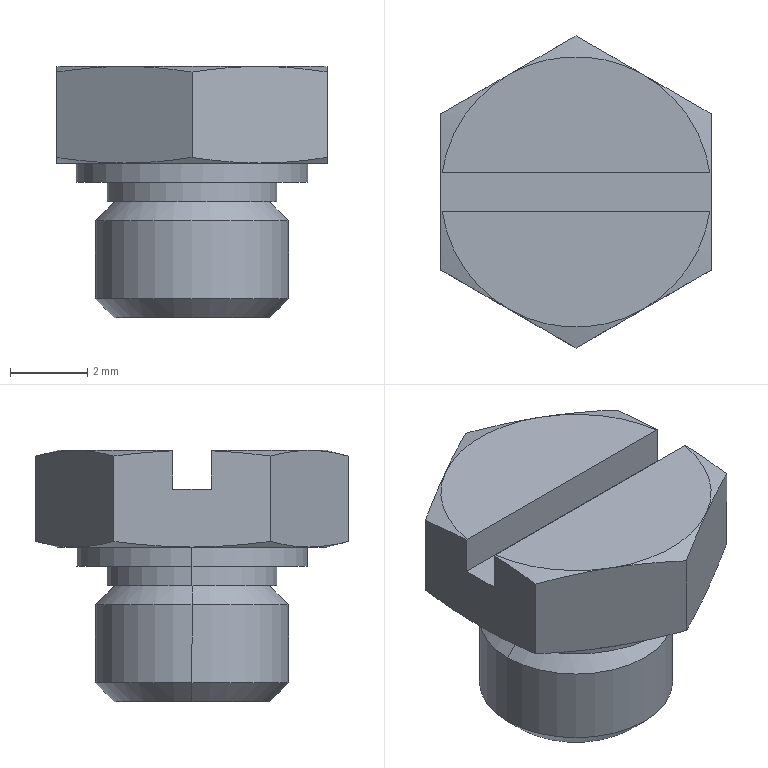Part | SolidWorks | features RefAxis 3, ICE 2, 3DProfileFeature 1, Revolution 1 | 1 solid | 37 faces | box 7 x 8.083 x 6.5 mm | volume 175.846 mm3 | cone 16 | plane 15 | cylinder 6 | commonest cylinder face diameters 4.4 x2 5 x2 6 x2
STEP:
#1=CARTESIAN_POINT('',(2.01,0.,-3.5));
#2=VERTEX_POINT('',#1);
#3=CARTESIAN_POINT('',(-2.01,0.,-3.5));
#4=VERTEX_POINT('',#3);
#5=CARTESIAN_POINT('',(0.,0.,-3.5));
#6=DIRECTION('',(0.,0.,1.));
#7=DIRECTION('',(1.,0.,0.));
#8=AXIS2_PLACEMENT_3D('',#5,#6,#7);
#9=CIRCLE('',#8,2.01);
#10=EDGE_CURVE('',#2,#4,#9,.T.);
#11=ORIENTED_EDGE('',*,*,#10,.T.);
#12=CARTESIAN_POINT('',(-2.5,0.,-3.01));
#13=VERTEX_POINT('',#12);
#14=CARTESIAN_POINT('',(-2.01,0.,-3.5));
#15=DIRECTION('',(-0.7071,0.,0.7071));
#16=VECTOR('',#15,1000.);
#17=LINE('',#14,#16);
#18=EDGE_CURVE('',#4,#13,#17,.T.);
#19=ORIENTED_EDGE('',*,*,#18,.T.);
#20=CARTESIAN_POINT('',(2.5,0.,-3.01));
#21=VERTEX_POINT('',#20);
#22=CARTESIAN_POINT('',(0.,0.,-3.01));
#23=DIRECTION('',(0.,0.,1.));
#24=DIRECTION('',(1.,0.,0.));
#25=AXIS2_PLACEMENT_3D('',#22,#23,#24);
#26=CIRCLE('',#25,2.5);
#27=EDGE_CURVE('',#21,#13,#26,.T.);
#28=ORIENTED_EDGE('',*,*,#27,.F.);
#29=CARTESIAN_POINT('',(2.01,0.,-3.5));
#30=DIRECTION('',(0.7071,0.,0.7071));
#31=VECTOR('',#30,1000.);
#32=LINE('',#29,#31);
#33=EDGE_CURVE('',#2,#21,#32,.T.);
#34=ORIENTED_EDGE('',*,*,#33,.F.);
#35=EDGE_LOOP('',(#11,#19,#28,#34));
#36=FACE_OUTER_BOUND('',#35,.T.);
#37=CARTESIAN_POINT('',(0.,0.,-3.5));
#38=DIRECTION('',(0.,0.,1.));
#39=DIRECTION('',(1.,0.,0.));
#40=AXIS2_PLACEMENT_3D('',#37,#38,#39);
#41=CONICAL_SURFACE('',#40,2.01,0.7854);
#42=ADVANCED_FACE('',(#36),#41,.T.);
#43=ORIENTED_EDGE('',*,*,#27,.T.);
#44=CARTESIAN_POINT('',(-2.5,0.,-0.9905));
#45=VERTEX_POINT('',#44);
#46=CARTESIAN_POINT('',(-2.5,0.,-3.5));
#47=DIRECTION('',(0.,0.,1.));
#48=VECTOR('',#47,1000.);
#49=LINE('',#46,#48);
#50=EDGE_CURVE('',#13,#45,#49,.T.);
#51=ORIENTED_EDGE('',*,*,#50,.T.);
#52=CARTESIAN_POINT('',(2.5,0.,-0.9905));
#53=VERTEX_POINT('',#52);
#54=CARTESIAN_POINT('',(0.,0.,-0.9905));
#55=DIRECTION('',(0.,0.,1.));
#56=DIRECTION('',(1.,0.,0.));
#57=AXIS2_PLACEMENT_3D('',#54,#55,#56);
#58=CIRCLE('',#57,2.5);
#59=EDGE_CURVE('',#53,#45,#58,.T.);
#60=ORIENTED_EDGE('',*,*,#59,.F.);
#61=CARTESIAN_POINT('',(2.5,0.,-3.5));
#62=DIRECTION('',(0.,0.,1.));
#63=VECTOR('',#62,1000.);
#64=LINE('',#61,#63);
#65=EDGE_CURVE('',#21,#53,#64,.T.);
#66=ORIENTED_EDGE('',*,*,#65,.F.);
#67=EDGE_LOOP('',(#43,#51,#60,#66));
#68=FACE_OUTER_BOUND('',#67,.T.);
#69=CARTESIAN_POINT('',(0.,0.,-3.5));
#70=DIRECTION('',(0.,0.,1.));
#71=DIRECTION('',(1.,0.,0.));
#72=AXIS2_PLACEMENT_3D('',#69,#70,#71);
#73=CYLINDRICAL_SURFACE('',#72,2.5);
#74=ADVANCED_FACE('',(#68),#73,.T.);
#75=CARTESIAN_POINT('',(2.01,0.,-0.5));
#76=VERTEX_POINT('',#75);
#77=CARTESIAN_POINT('',(-2.01,0.,-0.5));
#78=VERTEX_POINT('',#77);
#79=CARTESIAN_POINT('',(0.,0.,-0.5));
#80=DIRECTION('',(0.,0.,1.));
#81=DIRECTION('',(1.,0.,0.));
#82=AXIS2_PLACEMENT_3D('',#79,#80,#81);
#83=CIRCLE('',#82,2.01);
#84=EDGE_CURVE('',#76,#78,#83,.T.);
#85=ORIENTED_EDGE('',*,*,#84,.F.);
#86=CARTESIAN_POINT('',(2.5,0.,-0.9905));
#87=DIRECTION('',(0.7071,0.,-0.7071));
#88=VECTOR('',#87,1000.);
#89=LINE('',#86,#88);
#90=EDGE_CURVE('',#76,#53,#89,.T.);
#91=ORIENTED_EDGE('',*,*,#90,.T.);
#92=ORIENTED_EDGE('',*,*,#59,.T.);
#93=CARTESIAN_POINT('',(-2.5,0.,-0.9905));
#94=DIRECTION('',(-0.7071,0.,-0.7071));
#95=VECTOR('',#94,1000.);
#96=LINE('',#93,#95);
#97=EDGE_CURVE('',#78,#45,#96,.T.);
#98=ORIENTED_EDGE('',*,*,#97,.F.);
#99=EDGE_LOOP('',(#85,#91,#92,#98));
#100=FACE_OUTER_BOUND('',#99,.T.);
#101=CARTESIAN_POINT('',(0.,0.,-0.9905));
#102=DIRECTION('',(0.,0.,-1.));
#103=DIRECTION('',(-1.,0.,0.));
#104=AXIS2_PLACEMENT_3D('',#101,#102,#103);
#105=CONICAL_SURFACE('',#104,2.5,0.7854);
#106=ADVANCED_FACE('',(#100),#105,.T.);
#107=CARTESIAN_POINT('',(2.2,0.,-0.5));
#108=VERTEX_POINT('',#107);
#109=CARTESIAN_POINT('',(-2.2,0.,-0.5));
#110=VERTEX_POINT('',#109);
#111=CARTESIAN_POINT('',(0.,0.,-0.5));
#112=DIRECTION('',(0.,0.,1.));
#113=DIRECTION('',(1.,0.,0.));
#114=AXIS2_PLACEMENT_3D('',#111,#112,#113);
#115=CIRCLE('',#114,2.2);
#116=EDGE_CURVE('',#108,#110,#115,.T.);
#117=ORIENTED_EDGE('',*,*,#116,.T.);
#118=CARTESIAN_POINT('',(-2.2,0.,0.));
#119=VERTEX_POINT('',#118);
#120=CARTESIAN_POINT('',(-2.2,0.,-3.5));
#121=DIRECTION('',(0.,0.,1.));
#122=VECTOR('',#121,1000.);
#123=LINE('',#120,#122);
#124=EDGE_CURVE('',#110,#119,#123,.T.);
#125=ORIENTED_EDGE('',*,*,#124,.T.);
#126=CARTESIAN_POINT('',(2.2,0.,0.));
#127=VERTEX_POINT('',#126);
#128=CARTESIAN_POINT('',(0.,0.,0.));
#129=DIRECTION('',(0.,0.,1.));
#130=DIRECTION('',(1.,0.,0.));
#131=AXIS2_PLACEMENT_3D('',#128,#129,#130);
#132=CIRCLE('',#131,2.2);
#133=EDGE_CURVE('',#127,#119,#132,.T.);
#134=ORIENTED_EDGE('',*,*,#133,.F.);
#135=CARTESIAN_POINT('',(2.2,0.,-3.5));
#136=DIRECTION('',(0.,0.,1.));
#137=VECTOR('',#136,1000.);
#138=LINE('',#135,#137);
#139=EDGE_CURVE('',#108,#127,#138,.T.);
#140=ORIENTED_EDGE('',*,*,#139,.F.);
#141=EDGE_LOOP('',(#117,#125,#134,#140));
#142=FACE_OUTER_BOUND('',#141,.T.);
#143=CARTESIAN_POINT('',(0.,0.,-3.5));
#144=DIRECTION('',(0.,0.,1.));
#145=DIRECTION('',(1.,0.,0.));
#146=AXIS2_PLACEMENT_3D('',#143,#144,#145);
#147=CYLINDRICAL_SURFACE('',#146,2.2);
#148=ADVANCED_FACE('',(#142),#147,.T.);
#149=CARTESIAN_POINT('',(3.,0.,0.));
#150=VERTEX_POINT('',#149);
#151=CARTESIAN_POINT('',(-3.,0.,0.));
#152=VERTEX_POINT('',#151);
#153=CARTESIAN_POINT('',(0.,0.,0.));
#154=DIRECTION('',(0.,0.,1.));
#155=DIRECTION('',(1.,0.,0.));
#156=AXIS2_PLACEMENT_3D('',#153,#154,#155);
#157=CIRCLE('',#156,3.);
#158=EDGE_CURVE('',#150,#152,#157,.T.);
#159=ORIENTED_EDGE('',*,*,#158,.T.);
#160=CARTESIAN_POINT('',(-3.,0.,0.5));
#161=VERTEX_POINT('',#160);
#162=CARTESIAN_POINT('',(-3.,0.,-3.5));
#163=DIRECTION('',(0.,0.,1.));
#164=VECTOR('',#163,1000.);
#165=LINE('',#162,#164);
#166=EDGE_CURVE('',#152,#161,#165,.T.);
#167=ORIENTED_EDGE('',*,*,#166,.T.);
#168=CARTESIAN_POINT('',(3.,0.,0.5));
#169=VERTEX_POINT('',#168);
#170=CARTESIAN_POINT('',(0.,0.,0.5));
#171=DIRECTION('',(0.,0.,1.));
#172=DIRECTION('',(1.,0.,0.));
#173=AXIS2_PLACEMENT_3D('',#170,#171,#172);
#174=CIRCLE('',#173,3.);
#175=EDGE_CURVE('',#169,#161,#174,.T.);
#176=ORIENTED_EDGE('',*,*,#175,.F.);
#177=CARTESIAN_POINT('',(3.,0.,-3.5));
#178=DIRECTION('',(0.,0.,1.));
#179=VECTOR('',#178,1000.);
#180=LINE('',#177,#179);
#181=EDGE_CURVE('',#150,#169,#180,.T.);
#182=ORIENTED_EDGE('',*,*,#181,.F.);
#183=EDGE_LOOP('',(#159,#167,#176,#182));
#184=FACE_OUTER_BOUND('',#183,.T.);
#185=CARTESIAN_POINT('',(0.,0.,-3.5));
#186=DIRECTION('',(0.,0.,1.));
#187=DIRECTION('',(1.,0.,0.));
#188=AXIS2_PLACEMENT_3D('',#185,#186,#187);
#189=CYLINDRICAL_SURFACE('',#188,3.);
#190=ADVANCED_FACE('',(#184),#189,.T.);
#191=CARTESIAN_POINT('',(-1.75,3.031,3.));
#192=VERTEX_POINT('',#191);
#193=CARTESIAN_POINT('',(-3.464,0.5,3.));
#194=VERTEX_POINT('',#193);
#195=CARTESIAN_POINT('',(0.,0.,3.));
#196=DIRECTION('',(0.,0.,1.));
#197=DIRECTION('',(1.,0.,0.));
#198=AXIS2_PLACEMENT_3D('',#195,#196,#197);
#199=CIRCLE('',#198,3.5);
#200=EDGE_CURVE('',#192,#194,#199,.T.);
#201=ORIENTED_EDGE('',*,*,#200,.T.);
#202=CARTESIAN_POINT('',(3.464,0.5,3.));
#203=VERTEX_POINT('',#202);
#204=CARTESIAN_POINT('',(0.,0.5,3.));
#205=DIRECTION('',(1.,0.,0.));
#206=VECTOR('',#205,1000.);
#207=LINE('',#204,#206);
#208=EDGE_CURVE('',#194,#203,#207,.T.);
#209=ORIENTED_EDGE('',*,*,#208,.T.);
#210=CARTESIAN_POINT('',(1.75,3.031,3.));
#211=VERTEX_POINT('',#210);
#212=CARTESIAN_POINT('',(0.,0.,3.));
#213=DIRECTION('',(0.,0.,1.));
#214=DIRECTION('',(1.,0.,0.));
#215=AXIS2_PLACEMENT_3D('',#212,#213,#214);
#216=CIRCLE('',#215,3.5);
#217=EDGE_CURVE('',#203,#211,#216,.T.);
#218=ORIENTED_EDGE('',*,*,#217,.T.);
#219=CARTESIAN_POINT('',(0.,0.,3.));
#220=DIRECTION('',(0.,0.,1.));
#221=DIRECTION('',(1.,0.,0.));
#222=AXIS2_PLACEMENT_3D('',#219,#220,#221);
#223=CIRCLE('',#222,3.5);
#224=EDGE_CURVE('',#211,#192,#223,.T.);
#225=ORIENTED_EDGE('',*,*,#224,.T.);
#226=EDGE_LOOP('',(#201,#209,#218,#225));
#227=FACE_OUTER_BOUND('',#226,.T.);
#228=CARTESIAN_POINT('',(0.,0.,3.));
#229=DIRECTION('',(0.,0.,-1.));
#230=DIRECTION('',(-1.,0.,0.));
#231=AXIS2_PLACEMENT_3D('',#228,#229,#230);
#232=PLANE('',#231);
#233=ADVANCED_FACE('',(#227),#232,.F.);
#234=CARTESIAN_POINT('',(1.75,-3.031,0.5));
#235=VERTEX_POINT('',#234);
#236=CARTESIAN_POINT('',(0.,-4.041,0.6451));
#237=VERTEX_POINT('',#236);
#238=CARTESIAN_POINT('',(1.75,-3.031,0.5));
#239=CARTESIAN_POINT('',(1.167,-3.368,0.5));
#240=CARTESIAN_POINT('',(0.5833,-3.705,0.5548));
#241=CARTESIAN_POINT('',(0.,-4.041,0.6451));
#242=B_SPLINE_CURVE_WITH_KNOTS('',3,(#238,#239,#240,#241),.UNSPECIFIED.,.F.,.F.,(4,4),(0.002021,0.004042),.UNSPECIFIED.);
#243=EDGE_CURVE('',#235,#237,#242,.T.);
#244=ORIENTED_EDGE('',*,*,#243,.T.);
#245=CARTESIAN_POINT('',(-1.75,-3.031,0.5));
#246=VERTEX_POINT('',#245);
#247=CARTESIAN_POINT('',(0.,-4.041,0.6451));
#248=CARTESIAN_POINT('',(-0.5833,-3.705,0.5548));
#249=CARTESIAN_POINT('',(-1.167,-3.368,0.5));
#250=CARTESIAN_POINT('',(-1.75,-3.031,0.5));
#251=B_SPLINE_CURVE_WITH_KNOTS('',3,(#247,#248,#249,#250),.UNSPECIFIED.,.F.,.F.,(4,4),(0.000000231,0.002021),.UNSPECIFIED.);
#252=EDGE_CURVE('',#237,#246,#251,.T.);
#253=ORIENTED_EDGE('',*,*,#252,.T.);
#254=CARTESIAN_POINT('',(0.,0.,0.5));
#255=DIRECTION('',(0.,0.,1.));
#256=DIRECTION('',(1.,0.,0.));
#257=AXIS2_PLACEMENT_3D('',#254,#255,#256);
#258=CIRCLE('',#257,3.5);
#259=EDGE_CURVE('',#246,#235,#258,.T.);
#260=ORIENTED_EDGE('',*,*,#259,.T.);
#261=EDGE_LOOP('',(#244,#253,#260));
#262=FACE_OUTER_BOUND('',#261,.T.);
#263=CARTESIAN_POINT('',(0.,0.,0.5));
#264=DIRECTION('',(0.,0.,1.));
#265=DIRECTION('',(1.,0.,0.));
#266=AXIS2_PLACEMENT_3D('',#263,#264,#265);
#267=CONICAL_SURFACE('',#266,3.5,1.309);
#268=ADVANCED_FACE('',(#262),#267,.T.);
#269=CARTESIAN_POINT('',(-3.5,0.,0.5));
#270=VERTEX_POINT('',#269);
#271=CARTESIAN_POINT('',(0.,0.,0.5));
#272=DIRECTION('',(0.,0.,1.));
#273=DIRECTION('',(1.,0.,0.));
#274=AXIS2_PLACEMENT_3D('',#271,#272,#273);
#275=CIRCLE('',#274,3.5);
#276=EDGE_CURVE('',#270,#246,#275,.T.);
#277=ORIENTED_EDGE('',*,*,#276,.T.);
#278=CARTESIAN_POINT('',(-3.5,-2.021,0.6451));
#279=VERTEX_POINT('',#278);
#280=CARTESIAN_POINT('',(-1.75,-3.031,0.5));
#281=CARTESIAN_POINT('',(-2.333,-2.694,0.5));
#282=CARTESIAN_POINT('',(-2.917,-2.358,0.5548));
#283=CARTESIAN_POINT('',(-3.5,-2.021,0.6451));
#284=B_SPLINE_CURVE_WITH_KNOTS('',3,(#280,#281,#282,#283),.UNSPECIFIED.,.F.,.F.,(4,4),(0.002021,0.004042),.UNSPECIFIED.);
#285=EDGE_CURVE('',#246,#279,#284,.T.);
#286=ORIENTED_EDGE('',*,*,#285,.T.);
#287=CARTESIAN_POINT('',(-3.5,-2.021,0.6451));
#288=CARTESIAN_POINT('',(-3.5,-1.349,0.5551));
#289=CARTESIAN_POINT('',(-3.5,-0.6727,0.5));
#290=CARTESIAN_POINT('',(-3.5,0.,0.5));
#291=B_SPLINE_CURVE_WITH_KNOTS('',3,(#287,#288,#289,#290),.UNSPECIFIED.,.F.,.F.,(4,4),(0.0034,0.00543),.UNSPECIFIED.);
#292=EDGE_CURVE('',#279,#270,#291,.T.);
#293=ORIENTED_EDGE('',*,*,#292,.T.);
#294=EDGE_LOOP('',(#277,#286,#293));
#295=FACE_OUTER_BOUND('',#294,.T.);
#296=CARTESIAN_POINT('',(0.,0.,0.5));
#297=DIRECTION('',(0.,0.,1.));
#298=DIRECTION('',(1.,0.,0.));
#299=AXIS2_PLACEMENT_3D('',#296,#297,#298);
#300=CONICAL_SURFACE('',#299,3.5,1.309);
#301=ADVANCED_FACE('',(#295),#300,.T.);
#302=CARTESIAN_POINT('',(-1.75,3.031,0.5));
#303=VERTEX_POINT('',#302);
#304=CARTESIAN_POINT('',(0.,0.,0.5));
#305=DIRECTION('',(0.,0.,1.));
#306=DIRECTION('',(1.,0.,0.));
#307=AXIS2_PLACEMENT_3D('',#304,#305,#306);
#308=CIRCLE('',#307,3.5);
#309=EDGE_CURVE('',#303,#270,#308,.T.);
#310=ORIENTED_EDGE('',*,*,#309,.T.);
#311=CARTESIAN_POINT('',(-3.5,2.021,0.6451));
#312=VERTEX_POINT('',#311);
#313=CARTESIAN_POINT('',(-3.5,0.,0.5));
#314=CARTESIAN_POINT('',(-3.5,0.675,0.5));
#315=CARTESIAN_POINT('',(-3.5,1.348,0.555));
#316=CARTESIAN_POINT('',(-3.5,2.021,0.6451));
#317=B_SPLINE_CURVE_WITH_KNOTS('',3,(#313,#314,#315,#316),.UNSPECIFIED.,.F.,.F.,(4,4),(0.00543,0.007468),.UNSPECIFIED.);
#318=EDGE_CURVE('',#270,#312,#317,.T.);
#319=ORIENTED_EDGE('',*,*,#318,.T.);
#320=CARTESIAN_POINT('',(-3.5,2.021,0.6451));
#321=CARTESIAN_POINT('',(-2.917,2.358,0.5548));
#322=CARTESIAN_POINT('',(-2.333,2.694,0.5));
#323=CARTESIAN_POINT('',(-1.75,3.031,0.5));
#324=B_SPLINE_CURVE_WITH_KNOTS('',3,(#320,#321,#322,#323),.UNSPECIFIED.,.F.,.F.,(4,4),(0.000000231,0.002021),.UNSPECIFIED.);
#325=EDGE_CURVE('',#312,#303,#324,.T.);
#326=ORIENTED_EDGE('',*,*,#325,.T.);
#327=EDGE_LOOP('',(#310,#319,#326));
#328=FACE_OUTER_BOUND('',#327,.T.);
#329=CARTESIAN_POINT('',(0.,0.,0.5));
#330=DIRECTION('',(0.,0.,1.));
#331=DIRECTION('',(1.,0.,0.));
#332=AXIS2_PLACEMENT_3D('',#329,#330,#331);
#333=CONICAL_SURFACE('',#332,3.5,1.309);
#334=ADVANCED_FACE('',(#328),#333,.T.);
#335=CARTESIAN_POINT('',(3.5,0.,0.5));
#336=VERTEX_POINT('',#335);
#337=CARTESIAN_POINT('',(3.5,-2.021,0.6451));
#338=VERTEX_POINT('',#337);
#339=CARTESIAN_POINT('',(3.5,0.,0.5));
#340=CARTESIAN_POINT('',(3.5,-0.6727,0.5));
#341=CARTESIAN_POINT('',(3.5,-1.349,0.5551));
#342=CARTESIAN_POINT('',(3.5,-2.021,0.6451));
#343=B_SPLINE_CURVE_WITH_KNOTS('',3,(#339,#340,#341,#342),.UNSPECIFIED.,.F.,.F.,(4,4),(0.0098,0.01183),.UNSPECIFIED.);
#344=EDGE_CURVE('',#336,#338,#343,.T.);
#345=ORIENTED_EDGE('',*,*,#344,.T.);
#346=CARTESIAN_POINT('',(3.5,-2.021,0.6451));
#347=CARTESIAN_POINT('',(2.917,-2.358,0.5548));
#348=CARTESIAN_POINT('',(2.333,-2.694,0.5));
#349=CARTESIAN_POINT('',(1.75,-3.031,0.5));
#350=B_SPLINE_CURVE_WITH_KNOTS('',3,(#346,#347,#348,#349),.UNSPECIFIED.,.F.,.F.,(4,4),(0.000000231,0.002021),.UNSPECIFIED.);
#351=EDGE_CURVE('',#338,#235,#350,.T.);
#352=ORIENTED_EDGE('',*,*,#351,.T.);
#353=CARTESIAN_POINT('',(0.,0.,0.5));
#354=DIRECTION('',(0.,0.,1.));
#355=DIRECTION('',(1.,0.,0.));
#356=AXIS2_PLACEMENT_3D('',#353,#354,#355);
#357=CIRCLE('',#356,3.5);
#358=EDGE_CURVE('',#235,#336,#357,.T.);
#359=ORIENTED_EDGE('',*,*,#358,.T.);
#360=EDGE_LOOP('',(#345,#352,#359));
#361=FACE_OUTER_BOUND('',#360,.T.);
#362=CARTESIAN_POINT('',(0.,0.,0.5));
#363=DIRECTION('',(0.,0.,1.));
#364=DIRECTION('',(1.,0.,0.));
#365=AXIS2_PLACEMENT_3D('',#362,#363,#364);
#366=CONICAL_SURFACE('',#365,3.5,1.309);
#367=ADVANCED_FACE('',(#361),#366,.T.);
#368=CARTESIAN_POINT('',(1.75,3.031,0.5));
#369=VERTEX_POINT('',#368);
#370=CARTESIAN_POINT('',(0.,0.,0.5));
#371=DIRECTION('',(0.,0.,1.));
#372=DIRECTION('',(1.,0.,0.));
#373=AXIS2_PLACEMENT_3D('',#370,#371,#372);
#374=CIRCLE('',#373,3.5);
#375=EDGE_CURVE('',#369,#303,#374,.T.);
#376=ORIENTED_EDGE('',*,*,#375,.T.);
#377=CARTESIAN_POINT('',(0.,4.041,0.6451));
#378=VERTEX_POINT('',#377);
#379=CARTESIAN_POINT('',(-1.75,3.031,0.5));
#380=CARTESIAN_POINT('',(-1.167,3.368,0.5));
#381=CARTESIAN_POINT('',(-0.5833,3.705,0.5548));
#382=CARTESIAN_POINT('',(0.,4.041,0.6451));
#383=B_SPLINE_CURVE_WITH_KNOTS('',3,(#379,#380,#381,#382),.UNSPECIFIED.,.F.,.F.,(4,4),(0.002021,0.004042),.UNSPECIFIED.);
#384=EDGE_CURVE('',#303,#378,#383,.T.);
#385=ORIENTED_EDGE('',*,*,#384,.T.);
#386=CARTESIAN_POINT('',(0.,4.041,0.6451));
#387=CARTESIAN_POINT('',(0.5833,3.705,0.5548));
#388=CARTESIAN_POINT('',(1.167,3.368,0.5));
#389=CARTESIAN_POINT('',(1.75,3.031,0.5));
#390=B_SPLINE_CURVE_WITH_KNOTS('',3,(#386,#387,#388,#389),.UNSPECIFIED.,.F.,.F.,(4,4),(0.000000231,0.002021),.UNSPECIFIED.);
#391=EDGE_CURVE('',#378,#369,#390,.T.);
#392=ORIENTED_EDGE('',*,*,#391,.T.);
#393=EDGE_LOOP('',(#376,#385,#392));
#394=FACE_OUTER_BOUND('',#393,.T.);
#395=CARTESIAN_POINT('',(0.,0.,0.5));
#396=DIRECTION('',(0.,0.,1.));
#397=DIRECTION('',(1.,0.,0.));
#398=AXIS2_PLACEMENT_3D('',#395,#396,#397);
#399=CONICAL_SURFACE('',#398,3.5,1.309);
#400=ADVANCED_FACE('',(#394),#399,.T.);
#401=CARTESIAN_POINT('',(3.5,2.021,0.6451));
#402=VERTEX_POINT('',#401);
#403=CARTESIAN_POINT('',(1.75,3.031,0.5));
#404=CARTESIAN_POINT('',(2.333,2.694,0.5));
#405=CARTESIAN_POINT('',(2.917,2.358,0.5548));
#406=CARTESIAN_POINT('',(3.5,2.021,0.6451));
#407=B_SPLINE_CURVE_WITH_KNOTS('',3,(#403,#404,#405,#406),.UNSPECIFIED.,.F.,.F.,(4,4),(0.002021,0.004042),.UNSPECIFIED.);
#408=EDGE_CURVE('',#369,#402,#407,.T.);
#409=ORIENTED_EDGE('',*,*,#408,.T.);
#410=CARTESIAN_POINT('',(3.5,2.021,0.6451));
#411=CARTESIAN_POINT('',(3.5,1.348,0.555));
#412=CARTESIAN_POINT('',(3.5,0.675,0.5));
#413=CARTESIAN_POINT('',(3.5,0.,0.5));
#414=B_SPLINE_CURVE_WITH_KNOTS('',3,(#410,#411,#412,#413),.UNSPECIFIED.,.F.,.F.,(4,4),(0.007765,0.0098),.UNSPECIFIED.);
#415=EDGE_CURVE('',#402,#336,#414,.T.);
#416=ORIENTED_EDGE('',*,*,#415,.T.);
#417=CARTESIAN_POINT('',(0.,0.,0.5));
#418=DIRECTION('',(0.,0.,1.));
#419=DIRECTION('',(1.,0.,0.));
#420=AXIS2_PLACEMENT_3D('',#417,#418,#419);
#421=CIRCLE('',#420,3.5);
#422=EDGE_CURVE('',#336,#369,#421,.T.);
#423=ORIENTED_EDGE('',*,*,#422,.T.);
#424=EDGE_LOOP('',(#409,#416,#423));
#425=FACE_OUTER_BOUND('',#424,.T.);
#426=CARTESIAN_POINT('',(0.,0.,0.5));
#427=DIRECTION('',(0.,0.,1.));
#428=DIRECTION('',(1.,0.,0.));
#429=AXIS2_PLACEMENT_3D('',#426,#427,#428);
#430=CONICAL_SURFACE('',#429,3.5,1.309);
#431=ADVANCED_FACE('',(#425),#430,.T.);
#432=ORIENTED_EDGE('',*,*,#422,.F.);
#433=ORIENTED_EDGE('',*,*,#358,.F.);
#434=ORIENTED_EDGE('',*,*,#259,.F.);
#435=ORIENTED_EDGE('',*,*,#276,.F.);
#436=ORIENTED_EDGE('',*,*,#309,.F.);
#437=ORIENTED_EDGE('',*,*,#375,.F.);
#438=EDGE_LOOP('',(#432,#433,#434,#435,#436,#437));
#439=FACE_OUTER_BOUND('',#438,.T.);
#440=ORIENTED_EDGE('',*,*,#175,.T.);
#441=CARTESIAN_POINT('',(0.,0.,0.5));
#442=DIRECTION('',(0.,0.,1.));
#443=DIRECTION('',(1.,0.,0.));
#444=AXIS2_PLACEMENT_3D('',#441,#442,#443);
#445=CIRCLE('',#444,3.);
#446=EDGE_CURVE('',#161,#169,#445,.T.);
#447=ORIENTED_EDGE('',*,*,#446,.T.);
#448=EDGE_LOOP('',(#440,#447));
#449=FACE_BOUND('',#448,.T.);
#450=CARTESIAN_POINT('',(0.,3.5,0.5));
#451=DIRECTION('',(0.,0.,1.));
#452=DIRECTION('',(1.,0.,0.));
#453=AXIS2_PLACEMENT_3D('',#450,#451,#452);
#454=PLANE('',#453);
#455=ADVANCED_FACE('',(#439,#449),#454,.F.);
#456=ORIENTED_EDGE('',*,*,#166,.F.);
#457=CARTESIAN_POINT('',(0.,0.,0.));
#458=DIRECTION('',(0.,0.,1.));
#459=DIRECTION('',(1.,0.,0.));
#460=AXIS2_PLACEMENT_3D('',#457,#458,#459);
#461=CIRCLE('',#460,3.);
#462=EDGE_CURVE('',#152,#150,#461,.T.);
#463=ORIENTED_EDGE('',*,*,#462,.T.);
#464=ORIENTED_EDGE('',*,*,#181,.T.);
#465=ORIENTED_EDGE('',*,*,#446,.F.);
#466=EDGE_LOOP('',(#456,#463,#464,#465));
#467=FACE_OUTER_BOUND('',#466,.T.);
#468=CARTESIAN_POINT('',(0.,0.,-3.5));
#469=DIRECTION('',(0.,0.,1.));
#470=DIRECTION('',(1.,0.,0.));
#471=AXIS2_PLACEMENT_3D('',#468,#469,#470);
#472=CYLINDRICAL_SURFACE('',#471,3.);
#473=ADVANCED_FACE('',(#467),#472,.T.);
#474=ORIENTED_EDGE('',*,*,#158,.F.);
#475=ORIENTED_EDGE('',*,*,#462,.F.);
#476=EDGE_LOOP('',(#474,#475));
#477=FACE_OUTER_BOUND('',#476,.T.);
#478=ORIENTED_EDGE('',*,*,#133,.T.);
#479=CARTESIAN_POINT('',(0.,0.,0.));
#480=DIRECTION('',(0.,0.,1.));
#481=DIRECTION('',(1.,0.,0.));
#482=AXIS2_PLACEMENT_3D('',#479,#480,#481);
#483=CIRCLE('',#482,2.2);
#484=EDGE_CURVE('',#119,#127,#483,.T.);
#485=ORIENTED_EDGE('',*,*,#484,.T.);
#486=EDGE_LOOP('',(#478,#485));
#487=FACE_BOUND('',#486,.T.);
#488=CARTESIAN_POINT('',(0.,3.,0.));
#489=DIRECTION('',(0.,0.,1.));
#490=DIRECTION('',(1.,0.,0.));
#491=AXIS2_PLACEMENT_3D('',#488,#489,#490);
#492=PLANE('',#491);
#493=ADVANCED_FACE('',(#477,#487),#492,.F.);
#494=ORIENTED_EDGE('',*,*,#124,.F.);
#495=CARTESIAN_POINT('',(0.,0.,-0.5));
#496=DIRECTION('',(0.,0.,1.));
#497=DIRECTION('',(1.,0.,0.));
#498=AXIS2_PLACEMENT_3D('',#495,#496,#497);
#499=CIRCLE('',#498,2.2);
#500=EDGE_CURVE('',#110,#108,#499,.T.);
#501=ORIENTED_EDGE('',*,*,#500,.T.);
#502=ORIENTED_EDGE('',*,*,#139,.T.);
#503=ORIENTED_EDGE('',*,*,#484,.F.);
#504=EDGE_LOOP('',(#494,#501,#502,#503));
#505=FACE_OUTER_BOUND('',#504,.T.);
#506=CARTESIAN_POINT('',(0.,0.,-3.5));
#507=DIRECTION('',(0.,0.,1.));
#508=DIRECTION('',(1.,0.,0.));
#509=AXIS2_PLACEMENT_3D('',#506,#507,#508);
#510=CYLINDRICAL_SURFACE('',#509,2.2);
#511=ADVANCED_FACE('',(#505),#510,.T.);
#512=ORIENTED_EDGE('',*,*,#116,.F.);
#513=ORIENTED_EDGE('',*,*,#500,.F.);
#514=EDGE_LOOP('',(#512,#513));
#515=FACE_OUTER_BOUND('',#514,.T.);
#516=CARTESIAN_POINT('',(0.,0.,-0.5));
#517=DIRECTION('',(0.,0.,1.));
#518=DIRECTION('',(1.,0.,0.));
#519=AXIS2_PLACEMENT_3D('',#516,#517,#518);
#520=CIRCLE('',#519,2.01);
#521=EDGE_CURVE('',#78,#76,#520,.T.);
#522=ORIENTED_EDGE('',*,*,#521,.T.);
#523=ORIENTED_EDGE('',*,*,#84,.T.);
#524=EDGE_LOOP('',(#522,#523));
#525=FACE_BOUND('',#524,.T.);
#526=CARTESIAN_POINT('',(0.,2.2,-0.5));
#527=DIRECTION('',(0.,0.,1.));
#528=DIRECTION('',(1.,0.,0.));
#529=AXIS2_PLACEMENT_3D('',#526,#527,#528);
#530=PLANE('',#529);
#531=ADVANCED_FACE('',(#515,#525),#530,.F.);
#532=ORIENTED_EDGE('',*,*,#90,.F.);
#533=ORIENTED_EDGE('',*,*,#521,.F.);
#534=ORIENTED_EDGE('',*,*,#97,.T.);
#535=CARTESIAN_POINT('',(0.,0.,-0.9905));
#536=DIRECTION('',(0.,0.,1.));
#537=DIRECTION('',(1.,0.,0.));
#538=AXIS2_PLACEMENT_3D('',#535,#536,#537);
#539=CIRCLE('',#538,2.5);
#540=EDGE_CURVE('',#45,#53,#539,.T.);
#541=ORIENTED_EDGE('',*,*,#540,.T.);
#542=EDGE_LOOP('',(#532,#533,#534,#541));
#543=FACE_OUTER_BOUND('',#542,.T.);
#544=CARTESIAN_POINT('',(0.,0.,-0.9905));
#545=DIRECTION('',(0.,0.,-1.));
#546=DIRECTION('',(-1.,0.,0.));
#547=AXIS2_PLACEMENT_3D('',#544,#545,#546);
#548=CONICAL_SURFACE('',#547,2.5,0.7854);
#549=ADVANCED_FACE('',(#543),#548,.T.);
#550=ORIENTED_EDGE('',*,*,#50,.F.);
#551=CARTESIAN_POINT('',(0.,0.,-3.01));
#552=DIRECTION('',(0.,0.,1.));
#553=DIRECTION('',(1.,0.,0.));
#554=AXIS2_PLACEMENT_3D('',#551,#552,#553);
#555=CIRCLE('',#554,2.5);
#556=EDGE_CURVE('',#13,#21,#555,.T.);
#557=ORIENTED_EDGE('',*,*,#556,.T.);
#558=ORIENTED_EDGE('',*,*,#65,.T.);
#559=ORIENTED_EDGE('',*,*,#540,.F.);
#560=EDGE_LOOP('',(#550,#557,#558,#559));
#561=FACE_OUTER_BOUND('',#560,.T.);
#562=CARTESIAN_POINT('',(0.,0.,-3.5));
#563=DIRECTION('',(0.,0.,1.));
#564=DIRECTION('',(1.,0.,0.));
#565=AXIS2_PLACEMENT_3D('',#562,#563,#564);
#566=CYLINDRICAL_SURFACE('',#565,2.5);
#567=ADVANCED_FACE('',(#561),#566,.T.);
#568=ORIENTED_EDGE('',*,*,#18,.F.);
#569=CARTESIAN_POINT('',(0.,0.,-3.5));
#570=DIRECTION('',(0.,0.,1.));
#571=DIRECTION('',(1.,0.,0.));
#572=AXIS2_PLACEMENT_3D('',#569,#570,#571);
#573=CIRCLE('',#572,2.01);
#574=EDGE_CURVE('',#4,#2,#573,.T.);
#575=ORIENTED_EDGE('',*,*,#574,.T.);
#576=ORIENTED_EDGE('',*,*,#33,.T.);
#577=ORIENTED_EDGE('',*,*,#556,.F.);
#578=EDGE_LOOP('',(#568,#575,#576,#577));
#579=FACE_OUTER_BOUND('',#578,.T.);
#580=CARTESIAN_POINT('',(0.,0.,-3.5));
#581=DIRECTION('',(0.,0.,1.));
#582=DIRECTION('',(1.,0.,0.));
#583=AXIS2_PLACEMENT_3D('',#580,#581,#582);
#584=CONICAL_SURFACE('',#583,2.01,0.7854);
#585=ADVANCED_FACE('',(#579),#584,.T.);
#586=ORIENTED_EDGE('',*,*,#10,.F.);
#587=ORIENTED_EDGE('',*,*,#574,.F.);
#588=EDGE_LOOP('',(#586,#587));
#589=FACE_OUTER_BOUND('',#588,.T.);
#590=CARTESIAN_POINT('',(0.,2.01,-3.5));
#591=DIRECTION('',(0.,0.,1.));
#592=DIRECTION('',(1.,0.,0.));
#593=AXIS2_PLACEMENT_3D('',#590,#591,#592);
#594=PLANE('',#593);
#595=ADVANCED_FACE('',(#589),#594,.F.);
#596=CARTESIAN_POINT('',(0.,4.041,2.855));
#597=VERTEX_POINT('',#596);
#598=CARTESIAN_POINT('',(0.,4.041,3.));
#599=DIRECTION('',(0.,0.,-1.));
#600=VECTOR('',#599,1000.);
#601=LINE('',#598,#600);
#602=EDGE_CURVE('',#597,#378,#601,.T.);
#603=ORIENTED_EDGE('',*,*,#602,.T.);
#604=ORIENTED_EDGE('',*,*,#384,.F.);
#605=ORIENTED_EDGE('',*,*,#325,.F.);
#606=CARTESIAN_POINT('',(-3.5,2.021,2.855));
#607=VERTEX_POINT('',#606);
#608=CARTESIAN_POINT('',(-3.5,2.021,3.));
#609=DIRECTION('',(0.,0.,-1.));
#610=VECTOR('',#609,1000.);
#611=LINE('',#608,#610);
#612=EDGE_CURVE('',#607,#312,#611,.T.);
#613=ORIENTED_EDGE('',*,*,#612,.F.);
#614=CARTESIAN_POINT('',(-1.75,3.031,3.));
#615=CARTESIAN_POINT('',(-2.333,2.694,3.));
#616=CARTESIAN_POINT('',(-2.917,2.358,2.945));
#617=CARTESIAN_POINT('',(-3.5,2.021,2.855));
#618=B_SPLINE_CURVE_WITH_KNOTS('',3,(#614,#615,#616,#617),.UNSPECIFIED.,.F.,.F.,(4,4),(0.002021,0.004042),.UNSPECIFIED.);
#619=EDGE_CURVE('',#192,#607,#618,.T.);
#620=ORIENTED_EDGE('',*,*,#619,.F.);
#621=CARTESIAN_POINT('',(0.,4.041,2.855));
#622=CARTESIAN_POINT('',(-0.5833,3.705,2.945));
#623=CARTESIAN_POINT('',(-1.167,3.368,3.));
#624=CARTESIAN_POINT('',(-1.75,3.031,3.));
#625=B_SPLINE_CURVE_WITH_KNOTS('',3,(#621,#622,#623,#624),.UNSPECIFIED.,.F.,.F.,(4,4),(0.000000231,0.002021),.UNSPECIFIED.);
#626=EDGE_CURVE('',#597,#192,#625,.T.);
#627=ORIENTED_EDGE('',*,*,#626,.F.);
#628=EDGE_LOOP('',(#603,#604,#605,#613,#620,#627));
#629=FACE_OUTER_BOUND('',#628,.T.);
#630=CARTESIAN_POINT('',(0.,4.041,3.));
#631=DIRECTION('',(0.5,-0.866,0.));
#632=DIRECTION('',(0.866,0.5,0.));
#633=AXIS2_PLACEMENT_3D('',#630,#631,#632);
#634=PLANE('',#633);
#635=ADVANCED_FACE('',(#629),#634,.F.);
#636=CARTESIAN_POINT('',(-3.5,0.5,2.));
#637=VERTEX_POINT('',#636);
#638=CARTESIAN_POINT('',(-3.5,-0.5,2.));
#639=VERTEX_POINT('',#638);
#640=CARTESIAN_POINT('',(-3.5,2.021,2.));
#641=DIRECTION('',(0.,-1.,0.));
#642=VECTOR('',#641,1000.);
#643=LINE('',#640,#642);
#644=EDGE_CURVE('',#637,#639,#643,.T.);
#645=ORIENTED_EDGE('',*,*,#644,.F.);
#646=CARTESIAN_POINT('',(-3.5,0.5,2.99));
#647=VERTEX_POINT('',#646);
#648=CARTESIAN_POINT('',(-3.5,0.5,3.));
#649=DIRECTION('',(0.,0.,1.));
#650=VECTOR('',#649,1000.);
#651=LINE('',#648,#650);
#652=EDGE_CURVE('',#637,#647,#651,.T.);
#653=ORIENTED_EDGE('',*,*,#652,.T.);
#654=CARTESIAN_POINT('',(-3.5,2.021,2.855));
#655=CARTESIAN_POINT('',(-3.5,1.514,2.923));
#656=CARTESIAN_POINT('',(-3.5,1.008,2.971));
#657=CARTESIAN_POINT('',(-3.5,0.5,2.99));
#658=B_SPLINE_CURVE_WITH_KNOTS('',3,(#654,#655,#656,#657),.UNSPECIFIED.,.F.,.F.,(4,4),(0.007765,0.009297),.UNSPECIFIED.);
#659=EDGE_CURVE('',#607,#647,#658,.T.);
#660=ORIENTED_EDGE('',*,*,#659,.F.);
#661=ORIENTED_EDGE('',*,*,#612,.T.);
#662=ORIENTED_EDGE('',*,*,#318,.F.);
#663=ORIENTED_EDGE('',*,*,#292,.F.);
#664=CARTESIAN_POINT('',(-3.5,-2.021,2.855));
#665=VERTEX_POINT('',#664);
#666=CARTESIAN_POINT('',(-3.5,-2.021,3.));
#667=DIRECTION('',(0.,0.,-1.));
#668=VECTOR('',#667,1000.);
#669=LINE('',#666,#668);
#670=EDGE_CURVE('',#665,#279,#669,.T.);
#671=ORIENTED_EDGE('',*,*,#670,.F.);
#672=CARTESIAN_POINT('',(-3.5,-0.5,2.99));
#673=VERTEX_POINT('',#672);
#674=CARTESIAN_POINT('',(-3.5,-0.5,2.99));
#675=CARTESIAN_POINT('',(-3.5,-1.007,2.971));
#676=CARTESIAN_POINT('',(-3.5,-1.515,2.923));
#677=CARTESIAN_POINT('',(-3.5,-2.021,2.855));
#678=B_SPLINE_CURVE_WITH_KNOTS('',3,(#674,#675,#676,#677),.UNSPECIFIED.,.F.,.F.,(4,4),(0.0103,0.01183),.UNSPECIFIED.);
#679=EDGE_CURVE('',#673,#665,#678,.T.);
#680=ORIENTED_EDGE('',*,*,#679,.F.);
#681=CARTESIAN_POINT('',(-3.5,-0.5,3.));
#682=DIRECTION('',(0.,0.,-1.));
#683=VECTOR('',#682,1000.);
#684=LINE('',#681,#683);
#685=EDGE_CURVE('',#673,#639,#684,.T.);
#686=ORIENTED_EDGE('',*,*,#685,.T.);
#687=EDGE_LOOP('',(#645,#653,#660,#661,#662,#663,#671,#680,#686));
#688=FACE_OUTER_BOUND('',#687,.T.);
#689=CARTESIAN_POINT('',(-3.5,2.021,3.));
#690=DIRECTION('',(1.,0.,0.));
#691=DIRECTION('',(0.,0.,-1.));
#692=AXIS2_PLACEMENT_3D('',#689,#690,#691);
#693=PLANE('',#692);
#694=ADVANCED_FACE('',(#688),#693,.F.);
#695=ORIENTED_EDGE('',*,*,#670,.T.);
#696=ORIENTED_EDGE('',*,*,#285,.F.);
#697=ORIENTED_EDGE('',*,*,#252,.F.);
#698=CARTESIAN_POINT('',(0.,-4.041,2.855));
#699=VERTEX_POINT('',#698);
#700=CARTESIAN_POINT('',(0.,-4.041,3.));
#701=DIRECTION('',(0.,0.,-1.));
#702=VECTOR('',#701,1000.);
#703=LINE('',#700,#702);
#704=EDGE_CURVE('',#699,#237,#703,.T.);
#705=ORIENTED_EDGE('',*,*,#704,.F.);
#706=CARTESIAN_POINT('',(-1.75,-3.031,3.));
#707=VERTEX_POINT('',#706);
#708=CARTESIAN_POINT('',(-1.75,-3.031,3.));
#709=CARTESIAN_POINT('',(-1.167,-3.368,3.));
#710=CARTESIAN_POINT('',(-0.5833,-3.705,2.945));
#711=CARTESIAN_POINT('',(0.,-4.041,2.855));
#712=B_SPLINE_CURVE_WITH_KNOTS('',3,(#708,#709,#710,#711),.UNSPECIFIED.,.F.,.F.,(4,4),(0.002021,0.004042),.UNSPECIFIED.);
#713=EDGE_CURVE('',#707,#699,#712,.T.);
#714=ORIENTED_EDGE('',*,*,#713,.F.);
#715=CARTESIAN_POINT('',(-3.5,-2.021,2.855));
#716=CARTESIAN_POINT('',(-2.917,-2.358,2.945));
#717=CARTESIAN_POINT('',(-2.333,-2.694,3.));
#718=CARTESIAN_POINT('',(-1.75,-3.031,3.));
#719=B_SPLINE_CURVE_WITH_KNOTS('',3,(#715,#716,#717,#718),.UNSPECIFIED.,.F.,.F.,(4,4),(0.000000231,0.002021),.UNSPECIFIED.);
#720=EDGE_CURVE('',#665,#707,#719,.T.);
#721=ORIENTED_EDGE('',*,*,#720,.F.);
#722=EDGE_LOOP('',(#695,#696,#697,#705,#714,#721));
#723=FACE_OUTER_BOUND('',#722,.T.);
#724=CARTESIAN_POINT('',(-3.5,-2.021,3.));
#725=DIRECTION('',(0.5,0.866,0.));
#726=DIRECTION('',(-0.866,0.5,0.));
#727=AXIS2_PLACEMENT_3D('',#724,#725,#726);
#728=PLANE('',#727);
#729=ADVANCED_FACE('',(#723),#728,.F.);
#730=ORIENTED_EDGE('',*,*,#704,.T.);
#731=ORIENTED_EDGE('',*,*,#243,.F.);
#732=ORIENTED_EDGE('',*,*,#351,.F.);
#733=CARTESIAN_POINT('',(3.5,-2.021,2.855));
#734=VERTEX_POINT('',#733);
#735=CARTESIAN_POINT('',(3.5,-2.021,3.));
#736=DIRECTION('',(0.,0.,-1.));
#737=VECTOR('',#736,1000.);
#738=LINE('',#735,#737);
#739=EDGE_CURVE('',#734,#338,#738,.T.);
#740=ORIENTED_EDGE('',*,*,#739,.F.);
#741=CARTESIAN_POINT('',(1.75,-3.031,3.));
#742=VERTEX_POINT('',#741);
#743=CARTESIAN_POINT('',(1.75,-3.031,3.));
#744=CARTESIAN_POINT('',(2.333,-2.694,3.));
#745=CARTESIAN_POINT('',(2.917,-2.358,2.945));
#746=CARTESIAN_POINT('',(3.5,-2.021,2.855));
#747=B_SPLINE_CURVE_WITH_KNOTS('',3,(#743,#744,#745,#746),.UNSPECIFIED.,.F.,.F.,(4,4),(0.002021,0.004042),.UNSPECIFIED.);
#748=EDGE_CURVE('',#742,#734,#747,.T.);
#749=ORIENTED_EDGE('',*,*,#748,.F.);
#750=CARTESIAN_POINT('',(0.,-4.041,2.855));
#751=CARTESIAN_POINT('',(0.5833,-3.705,2.945));
#752=CARTESIAN_POINT('',(1.167,-3.368,3.));
#753=CARTESIAN_POINT('',(1.75,-3.031,3.));
#754=B_SPLINE_CURVE_WITH_KNOTS('',3,(#750,#751,#752,#753),.UNSPECIFIED.,.F.,.F.,(4,4),(0.000000231,0.002021),.UNSPECIFIED.);
#755=EDGE_CURVE('',#699,#742,#754,.T.);
#756=ORIENTED_EDGE('',*,*,#755,.F.);
#757=EDGE_LOOP('',(#730,#731,#732,#740,#749,#756));
#758=FACE_OUTER_BOUND('',#757,.T.);
#759=CARTESIAN_POINT('',(0.,-4.041,3.));
#760=DIRECTION('',(-0.5,0.866,0.));
#761=DIRECTION('',(-0.866,-0.5,0.));
#762=AXIS2_PLACEMENT_3D('',#759,#760,#761);
#763=PLANE('',#762);
#764=ADVANCED_FACE('',(#758),#763,.F.);
#765=CARTESIAN_POINT('',(3.5,0.5,2.99));
#766=VERTEX_POINT('',#765);
#767=CARTESIAN_POINT('',(3.5,2.021,2.855));
#768=VERTEX_POINT('',#767);
#769=CARTESIAN_POINT('',(3.5,0.5,2.99));
#770=CARTESIAN_POINT('',(3.5,1.008,2.971));
#771=CARTESIAN_POINT('',(3.5,1.514,2.923));
#772=CARTESIAN_POINT('',(3.5,2.021,2.855));
#773=B_SPLINE_CURVE_WITH_KNOTS('',3,(#769,#770,#771,#772),.UNSPECIFIED.,.F.,.F.,(4,4),(0.005933,0.007468),.UNSPECIFIED.);
#774=EDGE_CURVE('',#766,#768,#773,.T.);
#775=ORIENTED_EDGE('',*,*,#774,.F.);
#776=CARTESIAN_POINT('',(3.5,0.5,2.));
#777=VERTEX_POINT('',#776);
#778=CARTESIAN_POINT('',(3.5,0.5,3.));
#779=DIRECTION('',(0.,0.,-1.));
#780=VECTOR('',#779,1000.);
#781=LINE('',#778,#780);
#782=EDGE_CURVE('',#766,#777,#781,.T.);
#783=ORIENTED_EDGE('',*,*,#782,.T.);
#784=CARTESIAN_POINT('',(3.5,-0.5,2.));
#785=VERTEX_POINT('',#784);
#786=CARTESIAN_POINT('',(3.5,-2.021,2.));
#787=DIRECTION('',(0.,1.,0.));
#788=VECTOR('',#787,1000.);
#789=LINE('',#786,#788);
#790=EDGE_CURVE('',#785,#777,#789,.T.);
#791=ORIENTED_EDGE('',*,*,#790,.F.);
#792=CARTESIAN_POINT('',(3.5,-0.5,2.99));
#793=VERTEX_POINT('',#792);
#794=CARTESIAN_POINT('',(3.5,-0.5,3.));
#795=DIRECTION('',(0.,0.,1.));
#796=VECTOR('',#795,1000.);
#797=LINE('',#794,#796);
#798=EDGE_CURVE('',#785,#793,#797,.T.);
#799=ORIENTED_EDGE('',*,*,#798,.T.);
#800=CARTESIAN_POINT('',(3.5,-2.021,2.855));
#801=CARTESIAN_POINT('',(3.5,-1.515,2.923));
#802=CARTESIAN_POINT('',(3.5,-1.007,2.971));
#803=CARTESIAN_POINT('',(3.5,-0.5,2.99));
#804=B_SPLINE_CURVE_WITH_KNOTS('',3,(#800,#801,#802,#803),.UNSPECIFIED.,.F.,.F.,(4,4),(0.0034,0.004927),.UNSPECIFIED.);
#805=EDGE_CURVE('',#734,#793,#804,.T.);
#806=ORIENTED_EDGE('',*,*,#805,.F.);
#807=ORIENTED_EDGE('',*,*,#739,.T.);
#808=ORIENTED_EDGE('',*,*,#344,.F.);
#809=ORIENTED_EDGE('',*,*,#415,.F.);
#810=CARTESIAN_POINT('',(3.5,2.021,3.));
#811=DIRECTION('',(0.,0.,-1.));
#812=VECTOR('',#811,1000.);
#813=LINE('',#810,#812);
#814=EDGE_CURVE('',#768,#402,#813,.T.);
#815=ORIENTED_EDGE('',*,*,#814,.F.);
#816=EDGE_LOOP('',(#775,#783,#791,#799,#806,#807,#808,#809,#815));
#817=FACE_OUTER_BOUND('',#816,.T.);
#818=CARTESIAN_POINT('',(3.5,-2.021,3.));
#819=DIRECTION('',(-1.,0.,0.));
#820=DIRECTION('',(0.,0.,1.));
#821=AXIS2_PLACEMENT_3D('',#818,#819,#820);
#822=PLANE('',#821);
#823=ADVANCED_FACE('',(#817),#822,.F.);
#824=ORIENTED_EDGE('',*,*,#814,.T.);
#825=ORIENTED_EDGE('',*,*,#408,.F.);
#826=ORIENTED_EDGE('',*,*,#391,.F.);
#827=ORIENTED_EDGE('',*,*,#602,.F.);
#828=CARTESIAN_POINT('',(1.75,3.031,3.));
#829=CARTESIAN_POINT('',(1.167,3.368,3.));
#830=CARTESIAN_POINT('',(0.5833,3.705,2.945));
#831=CARTESIAN_POINT('',(0.,4.041,2.855));
#832=B_SPLINE_CURVE_WITH_KNOTS('',3,(#828,#829,#830,#831),.UNSPECIFIED.,.F.,.F.,(4,4),(0.002021,0.004042),.UNSPECIFIED.);
#833=EDGE_CURVE('',#211,#597,#832,.T.);
#834=ORIENTED_EDGE('',*,*,#833,.F.);
#835=CARTESIAN_POINT('',(3.5,2.021,2.855));
#836=CARTESIAN_POINT('',(2.917,2.358,2.945));
#837=CARTESIAN_POINT('',(2.333,2.694,3.));
#838=CARTESIAN_POINT('',(1.75,3.031,3.));
#839=B_SPLINE_CURVE_WITH_KNOTS('',3,(#835,#836,#837,#838),.UNSPECIFIED.,.F.,.F.,(4,4),(0.000000231,0.002021),.UNSPECIFIED.);
#840=EDGE_CURVE('',#768,#211,#839,.T.);
#841=ORIENTED_EDGE('',*,*,#840,.F.);
#842=EDGE_LOOP('',(#824,#825,#826,#827,#834,#841));
#843=FACE_OUTER_BOUND('',#842,.T.);
#844=CARTESIAN_POINT('',(3.5,2.021,3.));
#845=DIRECTION('',(-0.5,-0.866,0.));
#846=DIRECTION('',(0.866,-0.5,0.));
#847=AXIS2_PLACEMENT_3D('',#844,#845,#846);
#848=PLANE('',#847);
#849=ADVANCED_FACE('',(#843),#848,.F.);
#850=ORIENTED_EDGE('',*,*,#805,.T.);
#851=CARTESIAN_POINT('',(3.464,-0.5,3.));
#852=VERTEX_POINT('',#851);
#853=CARTESIAN_POINT('',(3.5,-0.5,2.99));
#854=CARTESIAN_POINT('',(3.488,-0.5,2.994));
#855=CARTESIAN_POINT('',(3.476,-0.5,2.997));
#856=CARTESIAN_POINT('',(3.464,-0.5,3.));
#857=B_SPLINE_CURVE_WITH_KNOTS('',3,(#853,#854,#855,#856),.UNSPECIFIED.,.F.,.F.,(4,4),(0.003091,0.003128),.UNSPECIFIED.);
#858=EDGE_CURVE('',#793,#852,#857,.T.);
#859=ORIENTED_EDGE('',*,*,#858,.T.);
#860=CARTESIAN_POINT('',(0.,0.,3.));
#861=DIRECTION('',(0.,0.,1.));
#862=DIRECTION('',(1.,0.,0.));
#863=AXIS2_PLACEMENT_3D('',#860,#861,#862);
#864=CIRCLE('',#863,3.5);
#865=EDGE_CURVE('',#742,#852,#864,.T.);
#866=ORIENTED_EDGE('',*,*,#865,.F.);
#867=ORIENTED_EDGE('',*,*,#748,.T.);
#868=EDGE_LOOP('',(#850,#859,#866,#867));
#869=FACE_OUTER_BOUND('',#868,.T.);
#870=CARTESIAN_POINT('',(0.,0.,2.598));
#871=DIRECTION('',(0.,0.,-1.));
#872=DIRECTION('',(-1.,0.,0.));
#873=AXIS2_PLACEMENT_3D('',#870,#871,#872);
#874=CONICAL_SURFACE('',#873,5.,1.309);
#875=ADVANCED_FACE('',(#869),#874,.T.);
#876=CARTESIAN_POINT('',(0.,0.,3.));
#877=DIRECTION('',(0.,0.,1.));
#878=DIRECTION('',(1.,0.,0.));
#879=AXIS2_PLACEMENT_3D('',#876,#877,#878);
#880=CIRCLE('',#879,3.5);
#881=EDGE_CURVE('',#707,#742,#880,.T.);
#882=ORIENTED_EDGE('',*,*,#881,.F.);
#883=ORIENTED_EDGE('',*,*,#713,.T.);
#884=ORIENTED_EDGE('',*,*,#755,.T.);
#885=EDGE_LOOP('',(#882,#883,#884));
#886=FACE_OUTER_BOUND('',#885,.T.);
#887=CARTESIAN_POINT('',(0.,0.,2.598));
#888=DIRECTION('',(0.,0.,-1.));
#889=DIRECTION('',(-1.,0.,0.));
#890=AXIS2_PLACEMENT_3D('',#887,#888,#889);
#891=CONICAL_SURFACE('',#890,5.,1.309);
#892=ADVANCED_FACE('',(#886),#891,.T.);
#893=CARTESIAN_POINT('',(-3.464,-0.5,3.));
#894=VERTEX_POINT('',#893);
#895=CARTESIAN_POINT('',(0.,0.,3.));
#896=DIRECTION('',(0.,0.,1.));
#897=DIRECTION('',(1.,0.,0.));
#898=AXIS2_PLACEMENT_3D('',#895,#896,#897);
#899=CIRCLE('',#898,3.5);
#900=EDGE_CURVE('',#894,#707,#899,.T.);
#901=ORIENTED_EDGE('',*,*,#900,.F.);
#902=CARTESIAN_POINT('',(-3.464,-0.5,3.));
#903=CARTESIAN_POINT('',(-3.476,-0.5,2.997));
#904=CARTESIAN_POINT('',(-3.488,-0.5,2.994));
#905=CARTESIAN_POINT('',(-3.5,-0.5,2.99));
#906=B_SPLINE_CURVE_WITH_KNOTS('',3,(#902,#903,#904,#905),.UNSPECIFIED.,.F.,.F.,(4,4),(0.003408,0.003445),.UNSPECIFIED.);
#907=EDGE_CURVE('',#894,#673,#906,.T.);
#908=ORIENTED_EDGE('',*,*,#907,.T.);
#909=ORIENTED_EDGE('',*,*,#679,.T.);
#910=ORIENTED_EDGE('',*,*,#720,.T.);
#911=EDGE_LOOP('',(#901,#908,#909,#910));
#912=FACE_OUTER_BOUND('',#911,.T.);
#913=CARTESIAN_POINT('',(0.,0.,2.598));
#914=DIRECTION('',(0.,0.,-1.));
#915=DIRECTION('',(-1.,0.,0.));
#916=AXIS2_PLACEMENT_3D('',#913,#914,#915);
#917=CONICAL_SURFACE('',#916,5.,1.309);
#918=ADVANCED_FACE('',(#912),#917,.T.);
#919=ORIENTED_EDGE('',*,*,#659,.T.);
#920=CARTESIAN_POINT('',(-3.5,0.5,2.99));
#921=CARTESIAN_POINT('',(-3.488,0.5,2.994));
#922=CARTESIAN_POINT('',(-3.476,0.5,2.997));
#923=CARTESIAN_POINT('',(-3.464,0.5,3.));
#924=B_SPLINE_CURVE_WITH_KNOTS('',3,(#920,#921,#922,#923),.UNSPECIFIED.,.F.,.F.,(4,4),(0.003091,0.003128),.UNSPECIFIED.);
#925=EDGE_CURVE('',#647,#194,#924,.T.);
#926=ORIENTED_EDGE('',*,*,#925,.T.);
#927=ORIENTED_EDGE('',*,*,#200,.F.);
#928=ORIENTED_EDGE('',*,*,#619,.T.);
#929=EDGE_LOOP('',(#919,#926,#927,#928));
#930=FACE_OUTER_BOUND('',#929,.T.);
#931=CARTESIAN_POINT('',(0.,0.,2.598));
#932=DIRECTION('',(0.,0.,-1.));
#933=DIRECTION('',(-1.,0.,0.));
#934=AXIS2_PLACEMENT_3D('',#931,#932,#933);
#935=CONICAL_SURFACE('',#934,5.,1.309);
#936=ADVANCED_FACE('',(#930),#935,.T.);
#937=ORIENTED_EDGE('',*,*,#217,.F.);
#938=CARTESIAN_POINT('',(3.464,0.5,3.));
#939=CARTESIAN_POINT('',(3.476,0.5,2.997));
#940=CARTESIAN_POINT('',(3.488,0.5,2.994));
#941=CARTESIAN_POINT('',(3.5,0.5,2.99));
#942=B_SPLINE_CURVE_WITH_KNOTS('',3,(#938,#939,#940,#941),.UNSPECIFIED.,.F.,.F.,(4,4),(0.003408,0.003445),.UNSPECIFIED.);
#943=EDGE_CURVE('',#203,#766,#942,.T.);
#944=ORIENTED_EDGE('',*,*,#943,.T.);
#945=ORIENTED_EDGE('',*,*,#774,.T.);
#946=ORIENTED_EDGE('',*,*,#840,.T.);
#947=EDGE_LOOP('',(#937,#944,#945,#946));
#948=FACE_OUTER_BOUND('',#947,.T.);
#949=CARTESIAN_POINT('',(0.,0.,2.598));
#950=DIRECTION('',(0.,0.,-1.));
#951=DIRECTION('',(-1.,0.,0.));
#952=AXIS2_PLACEMENT_3D('',#949,#950,#951);
#953=CONICAL_SURFACE('',#952,5.,1.309);
#954=ADVANCED_FACE('',(#948),#953,.T.);
#955=ORIENTED_EDGE('',*,*,#865,.T.);
#956=CARTESIAN_POINT('',(0.,-0.5,3.));
#957=DIRECTION('',(-1.,0.,0.));
#958=VECTOR('',#957,1000.);
#959=LINE('',#956,#958);
#960=EDGE_CURVE('',#852,#894,#959,.T.);
#961=ORIENTED_EDGE('',*,*,#960,.T.);
#962=ORIENTED_EDGE('',*,*,#900,.T.);
#963=ORIENTED_EDGE('',*,*,#881,.T.);
#964=EDGE_LOOP('',(#955,#961,#962,#963));
#965=FACE_OUTER_BOUND('',#964,.T.);
#966=CARTESIAN_POINT('',(0.,0.,3.));
#967=DIRECTION('',(0.,0.,-1.));
#968=DIRECTION('',(-1.,0.,0.));
#969=AXIS2_PLACEMENT_3D('',#966,#967,#968);
#970=PLANE('',#969);
#971=ADVANCED_FACE('',(#965),#970,.F.);
#972=ORIENTED_EDGE('',*,*,#833,.T.);
#973=ORIENTED_EDGE('',*,*,#626,.T.);
#974=ORIENTED_EDGE('',*,*,#224,.F.);
#975=EDGE_LOOP('',(#972,#973,#974));
#976=FACE_OUTER_BOUND('',#975,.T.);
#977=CARTESIAN_POINT('',(0.,0.,2.598));
#978=DIRECTION('',(0.,0.,-1.));
#979=DIRECTION('',(-1.,0.,0.));
#980=AXIS2_PLACEMENT_3D('',#977,#978,#979);
#981=CONICAL_SURFACE('',#980,5.,1.309);
#982=ADVANCED_FACE('',(#976),#981,.T.);
#983=ORIENTED_EDGE('',*,*,#644,.T.);
#984=CARTESIAN_POINT('',(-5.,-0.5,2.));
#985=DIRECTION('',(1.,0.,0.));
#986=VECTOR('',#985,1000.);
#987=LINE('',#984,#986);
#988=EDGE_CURVE('',#639,#785,#987,.T.);
#989=ORIENTED_EDGE('',*,*,#988,.T.);
#990=ORIENTED_EDGE('',*,*,#790,.T.);
#991=CARTESIAN_POINT('',(5.,0.5,2.));
#992=DIRECTION('',(-1.,0.,0.));
#993=VECTOR('',#992,1000.);
#994=LINE('',#991,#993);
#995=EDGE_CURVE('',#777,#637,#994,.T.);
#996=ORIENTED_EDGE('',*,*,#995,.T.);
#997=EDGE_LOOP('',(#983,#989,#990,#996));
#998=FACE_OUTER_BOUND('',#997,.T.);
#999=CARTESIAN_POINT('',(0.,0.,2.));
#1000=DIRECTION('',(0.,0.,1.));
#1001=DIRECTION('',(1.,0.,0.));
#1002=AXIS2_PLACEMENT_3D('',#999,#1000,#1001);
#1003=PLANE('',#1002);
#1004=ADVANCED_FACE('',(#998),#1003,.T.);
#1005=ORIENTED_EDGE('',*,*,#995,.F.);
#1006=ORIENTED_EDGE('',*,*,#782,.F.);
#1007=ORIENTED_EDGE('',*,*,#943,.F.);
#1008=ORIENTED_EDGE('',*,*,#208,.F.);
#1009=ORIENTED_EDGE('',*,*,#925,.F.);
#1010=ORIENTED_EDGE('',*,*,#652,.F.);
#1011=EDGE_LOOP('',(#1005,#1006,#1007,#1008,#1009,#1010));
#1012=FACE_OUTER_BOUND('',#1011,.T.);
#1013=CARTESIAN_POINT('',(5.,0.5,2.));
#1014=DIRECTION('',(0.,1.,0.));
#1015=DIRECTION('',(0.,0.,1.));
#1016=AXIS2_PLACEMENT_3D('',#1013,#1014,#1015);
#1017=PLANE('',#1016);
#1018=ADVANCED_FACE('',(#1012),#1017,.F.);
#1019=ORIENTED_EDGE('',*,*,#988,.F.);
#1020=ORIENTED_EDGE('',*,*,#685,.F.);
#1021=ORIENTED_EDGE('',*,*,#907,.F.);
#1022=ORIENTED_EDGE('',*,*,#960,.F.);
#1023=ORIENTED_EDGE('',*,*,#858,.F.);
#1024=ORIENTED_EDGE('',*,*,#798,.F.);
#1025=EDGE_LOOP('',(#1019,#1020,#1021,#1022,#1023,#1024));
#1026=FACE_OUTER_BOUND('',#1025,.T.);
#1027=CARTESIAN_POINT('',(-5.,-0.5,2.));
#1028=DIRECTION('',(0.,-1.,0.));
#1029=DIRECTION('',(0.,0.,-1.));
#1030=AXIS2_PLACEMENT_3D('',#1027,#1028,#1029);
#1031=PLANE('',#1030);
#1032=ADVANCED_FACE('',(#1026),#1031,.F.);
#1033=CLOSED_SHELL('',(#42,#74,#106,#148,#190,#233,#268,#301,#334,#367,#400,#431,#455,#473,#493,#511,#531,#549,#567,#585,#595,#635,#694,#729,#764,#823,#849,#875,#892,#918,#936,#954,#971,#982,#1004,#1018,#1032));
#1034=MANIFOLD_SOLID_BREP('',#1033);
#1035=CARTESIAN_POINT('',(0.,0.,0.));
#1036=DIRECTION('',(0.,0.,1.));
#1037=DIRECTION('',(1.,0.,0.));
#1038=AXIS2_PLACEMENT_3D('',#1035,#1036,#1037);
#1039=(LENGTH_UNIT()NAMED_UNIT(*)SI_UNIT(.MILLI.,.METRE.));
#1040=UNCERTAINTY_MEASURE_WITH_UNIT(LENGTH_MEASURE(0.00001),#1039,'','');
#1041=(NAMED_UNIT(*)PLANE_ANGLE_UNIT()SI_UNIT($,.RADIAN.));
#1042=(NAMED_UNIT(*)SI_UNIT($,.STERADIAN.)SOLID_ANGLE_UNIT());
#1043=(GEOMETRIC_REPRESENTATION_CONTEXT(3)GLOBAL_UNCERTAINTY_ASSIGNED_CONTEXT((#1040))GLOBAL_UNIT_ASSIGNED_CONTEXT((#1039,#1041,#1042))REPRESENTATION_CONTEXT('',''));
#1044=ADVANCED_BREP_SHAPE_REPRESENTATION('',(#1034,#1038),#1043);